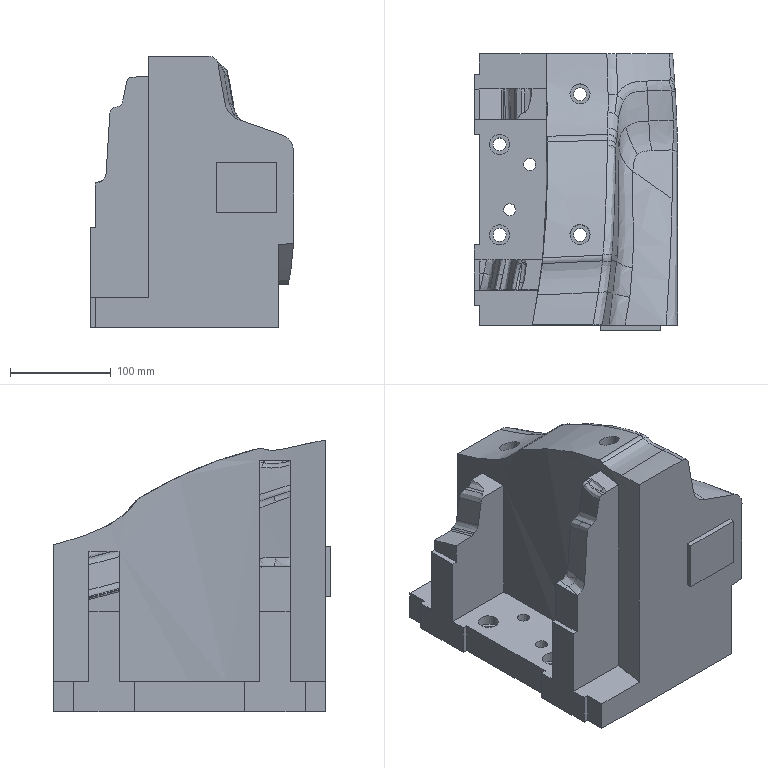Part | NX | features solid 2 | 1 solid | 119 faces | box 202 x 275 x 270.519 mm | volume 7893606 mm3 | spline 75 | plane 34 | cylinder 10 | commonest cylinder face diameters 13 x4 20 x4 12 x2